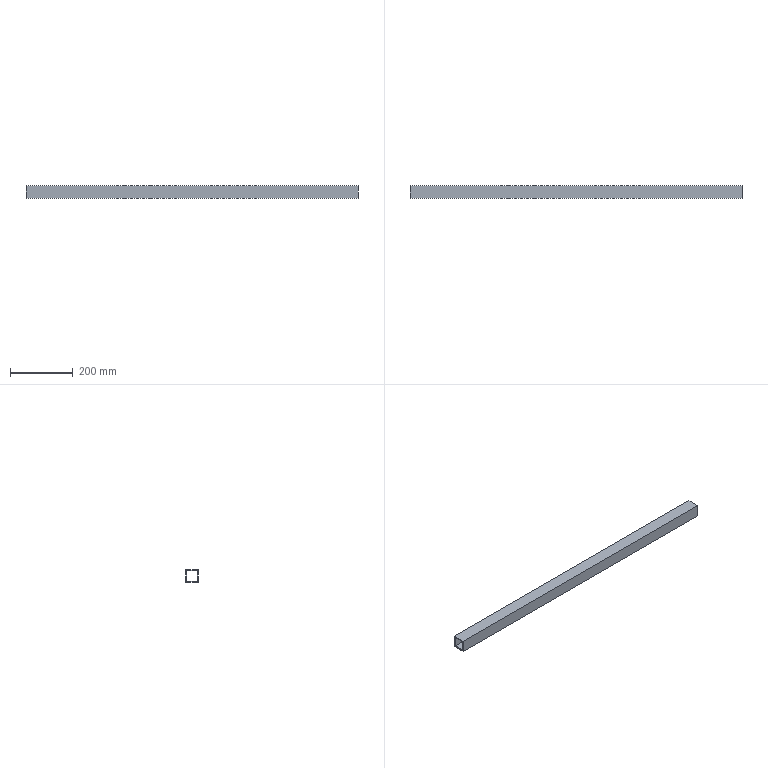Part | NX | features solid 2 | 1 solid | 10 faces | box 1060 x 40 x 40 mm | volume 610560 mm3 | plane 10
STEP:
#1=CARTESIAN_POINT('',(-1540.,-60.,-85.));
#2=VERTEX_POINT('',#1);
#3=CARTESIAN_POINT('',(-480.,-60.,-85.));
#4=VERTEX_POINT('',#3);
#5=CARTESIAN_POINT('',(119.393,-60.,-85.));
#6=DIRECTION('',(1.,0.,0.));
#7=VECTOR('',#6,1000.);
#8=LINE('',#5,#7);
#9=EDGE_CURVE('',#2,#4,#8,.T.);
#10=ORIENTED_EDGE('',*,*,#9,.T.);
#11=CARTESIAN_POINT('',(-480.,-60.,-45.));
#12=VERTEX_POINT('',#11);
#13=CARTESIAN_POINT('',(-480.,-60.,-70.));
#14=DIRECTION('',(0.,0.,1.));
#15=VECTOR('',#14,1000.);
#16=LINE('',#13,#15);
#17=EDGE_CURVE('',#4,#12,#16,.T.);
#18=ORIENTED_EDGE('',*,*,#17,.T.);
#19=CARTESIAN_POINT('',(-1540.,-60.,-45.));
#20=VERTEX_POINT('',#19);
#21=CARTESIAN_POINT('',(204.393,-60.,-45.));
#22=DIRECTION('',(1.,0.,0.));
#23=VECTOR('',#22,1000.);
#24=LINE('',#21,#23);
#25=EDGE_CURVE('',#20,#12,#24,.T.);
#26=ORIENTED_EDGE('',*,*,#25,.F.);
#27=CARTESIAN_POINT('',(-1540.,-60.,-70.));
#28=DIRECTION('',(0.,0.,-1.));
#29=VECTOR('',#28,1000.);
#30=LINE('',#27,#29);
#31=EDGE_CURVE('',#20,#2,#30,.T.);
#32=ORIENTED_EDGE('',*,*,#31,.T.);
#33=EDGE_LOOP('',(#10,#18,#26,#32));
#34=FACE_BOUND('',#33,.T.);
#35=CARTESIAN_POINT('',(119.393,-60.,-70.));
#36=DIRECTION('',(0.,1.,0.));
#37=DIRECTION('',(0.,0.,1.));
#38=AXIS2_PLACEMENT_3D('',#35,#36,#37);
#39=PLANE('',#38);
#40=ADVANCED_FACE('',(#34),#39,.F.);
#41=CARTESIAN_POINT('',(-1540.,-20.,-85.));
#42=VERTEX_POINT('',#41);
#43=CARTESIAN_POINT('',(-480.,-20.,-85.));
#44=VERTEX_POINT('',#43);
#45=CARTESIAN_POINT('',(204.393,-20.,-85.));
#46=DIRECTION('',(1.,0.,0.));
#47=VECTOR('',#46,1000.);
#48=LINE('',#45,#47);
#49=EDGE_CURVE('',#42,#44,#48,.T.);
#50=ORIENTED_EDGE('',*,*,#49,.T.);
#51=CARTESIAN_POINT('',(-480.,-640.,-85.));
#52=DIRECTION('',(0.,-1.,0.));
#53=VECTOR('',#52,1000.);
#54=LINE('',#51,#53);
#55=EDGE_CURVE('',#44,#4,#54,.T.);
#56=ORIENTED_EDGE('',*,*,#55,.T.);
#57=ORIENTED_EDGE('',*,*,#9,.F.);
#58=CARTESIAN_POINT('',(-1540.,-640.,-85.));
#59=DIRECTION('',(0.,1.,0.));
#60=VECTOR('',#59,1000.);
#61=LINE('',#58,#60);
#62=EDGE_CURVE('',#2,#42,#61,.T.);
#63=ORIENTED_EDGE('',*,*,#62,.T.);
#64=EDGE_LOOP('',(#50,#56,#57,#63));
#65=FACE_BOUND('',#64,.T.);
#66=CARTESIAN_POINT('',(204.393,-640.,-85.));
#67=DIRECTION('',(0.,0.,1.));
#68=DIRECTION('',(0.,-1.,0.));
#69=AXIS2_PLACEMENT_3D('',#66,#67,#68);
#70=PLANE('',#69);
#71=ADVANCED_FACE('',(#65),#70,.F.);
#72=ORIENTED_EDGE('',*,*,#25,.T.);
#73=CARTESIAN_POINT('',(-480.,-20.,-45.));
#74=VERTEX_POINT('',#73);
#75=CARTESIAN_POINT('',(-480.,-680.,-45.));
#76=DIRECTION('',(0.,1.,0.));
#77=VECTOR('',#76,1000.);
#78=LINE('',#75,#77);
#79=EDGE_CURVE('',#12,#74,#78,.T.);
#80=ORIENTED_EDGE('',*,*,#79,.T.);
#81=CARTESIAN_POINT('',(-1540.,-20.,-45.));
#82=VERTEX_POINT('',#81);
#83=CARTESIAN_POINT('',(204.393,-20.,-45.));
#84=DIRECTION('',(-1.,0.,0.));
#85=VECTOR('',#84,1000.);
#86=LINE('',#83,#85);
#87=EDGE_CURVE('',#74,#82,#86,.T.);
#88=ORIENTED_EDGE('',*,*,#87,.T.);
#89=CARTESIAN_POINT('',(-1540.,-680.,-45.));
#90=DIRECTION('',(0.,-1.,0.));
#91=VECTOR('',#90,1000.);
#92=LINE('',#89,#91);
#93=EDGE_CURVE('',#82,#20,#92,.T.);
#94=ORIENTED_EDGE('',*,*,#93,.T.);
#95=EDGE_LOOP('',(#72,#80,#88,#94));
#96=FACE_BOUND('',#95,.T.);
#97=CARTESIAN_POINT('',(204.393,-680.,-45.));
#98=DIRECTION('',(0.,0.,-1.));
#99=DIRECTION('',(0.,1.,0.));
#100=AXIS2_PLACEMENT_3D('',#97,#98,#99);
#101=PLANE('',#100);
#102=ADVANCED_FACE('',(#96),#101,.F.);
#103=ORIENTED_EDGE('',*,*,#87,.F.);
#104=CARTESIAN_POINT('',(-480.,-20.,-40.));
#105=DIRECTION('',(0.,0.,-1.));
#106=VECTOR('',#105,1000.);
#107=LINE('',#104,#106);
#108=EDGE_CURVE('',#74,#44,#107,.T.);
#109=ORIENTED_EDGE('',*,*,#108,.T.);
#110=ORIENTED_EDGE('',*,*,#49,.F.);
#111=CARTESIAN_POINT('',(-1540.,-20.,-40.));
#112=DIRECTION('',(0.,0.,1.));
#113=VECTOR('',#112,1000.);
#114=LINE('',#111,#113);
#115=EDGE_CURVE('',#42,#82,#114,.T.);
#116=ORIENTED_EDGE('',*,*,#115,.T.);
#117=EDGE_LOOP('',(#103,#109,#110,#116));
#118=FACE_BOUND('',#117,.T.);
#119=CARTESIAN_POINT('',(119.393,-20.,-40.));
#120=DIRECTION('',(0.,-1.,0.));
#121=DIRECTION('',(0.,0.,-1.));
#122=AXIS2_PLACEMENT_3D('',#119,#120,#121);
#123=PLANE('',#122);
#124=ADVANCED_FACE('',(#118),#123,.F.);
#125=CARTESIAN_POINT('',(-480.,-56.,-81.));
#126=VERTEX_POINT('',#125);
#127=CARTESIAN_POINT('',(-480.,-56.,-49.));
#128=VERTEX_POINT('',#127);
#129=CARTESIAN_POINT('',(-480.,-56.,-70.));
#130=DIRECTION('',(0.,0.,1.));
#131=VECTOR('',#130,1000.);
#132=LINE('',#129,#131);
#133=EDGE_CURVE('',#126,#128,#132,.T.);
#134=ORIENTED_EDGE('',*,*,#133,.F.);
#135=CARTESIAN_POINT('',(-1540.,-56.,-81.));
#136=VERTEX_POINT('',#135);
#137=CARTESIAN_POINT('',(119.393,-56.,-81.));
#138=DIRECTION('',(1.,0.,0.));
#139=VECTOR('',#138,1000.);
#140=LINE('',#137,#139);
#141=EDGE_CURVE('',#136,#126,#140,.T.);
#142=ORIENTED_EDGE('',*,*,#141,.F.);
#143=CARTESIAN_POINT('',(-1540.,-56.,-49.));
#144=VERTEX_POINT('',#143);
#145=CARTESIAN_POINT('',(-1540.,-56.,-70.));
#146=DIRECTION('',(0.,0.,-1.));
#147=VECTOR('',#146,1000.);
#148=LINE('',#145,#147);
#149=EDGE_CURVE('',#144,#136,#148,.T.);
#150=ORIENTED_EDGE('',*,*,#149,.F.);
#151=CARTESIAN_POINT('',(204.393,-56.,-49.));
#152=DIRECTION('',(1.,0.,0.));
#153=VECTOR('',#152,1000.);
#154=LINE('',#151,#153);
#155=EDGE_CURVE('',#144,#128,#154,.T.);
#156=ORIENTED_EDGE('',*,*,#155,.T.);
#157=EDGE_LOOP('',(#134,#142,#150,#156));
#158=FACE_BOUND('',#157,.T.);
#159=CARTESIAN_POINT('',(119.393,-56.,-70.));
#160=DIRECTION('',(0.,1.,0.));
#161=DIRECTION('',(0.,0.,1.));
#162=AXIS2_PLACEMENT_3D('',#159,#160,#161);
#163=PLANE('',#162);
#164=ADVANCED_FACE('',(#158),#163,.T.);
#165=CARTESIAN_POINT('',(-480.,-24.,-81.));
#166=VERTEX_POINT('',#165);
#167=CARTESIAN_POINT('',(-480.,-640.,-81.));
#168=DIRECTION('',(0.,-1.,0.));
#169=VECTOR('',#168,1000.);
#170=LINE('',#167,#169);
#171=EDGE_CURVE('',#166,#126,#170,.T.);
#172=ORIENTED_EDGE('',*,*,#171,.F.);
#173=CARTESIAN_POINT('',(-1540.,-24.,-81.));
#174=VERTEX_POINT('',#173);
#175=CARTESIAN_POINT('',(204.393,-24.,-81.));
#176=DIRECTION('',(1.,0.,0.));
#177=VECTOR('',#176,1000.);
#178=LINE('',#175,#177);
#179=EDGE_CURVE('',#174,#166,#178,.T.);
#180=ORIENTED_EDGE('',*,*,#179,.F.);
#181=CARTESIAN_POINT('',(-1540.,-640.,-81.));
#182=DIRECTION('',(0.,1.,0.));
#183=VECTOR('',#182,1000.);
#184=LINE('',#181,#183);
#185=EDGE_CURVE('',#136,#174,#184,.T.);
#186=ORIENTED_EDGE('',*,*,#185,.F.);
#187=ORIENTED_EDGE('',*,*,#141,.T.);
#188=EDGE_LOOP('',(#172,#180,#186,#187));
#189=FACE_BOUND('',#188,.T.);
#190=CARTESIAN_POINT('',(204.393,-640.,-81.));
#191=DIRECTION('',(0.,0.,1.));
#192=DIRECTION('',(0.,-1.,0.));
#193=AXIS2_PLACEMENT_3D('',#190,#191,#192);
#194=PLANE('',#193);
#195=ADVANCED_FACE('',(#189),#194,.T.);
#196=CARTESIAN_POINT('',(-480.,-24.,-49.));
#197=VERTEX_POINT('',#196);
#198=CARTESIAN_POINT('',(-480.,-680.,-49.));
#199=DIRECTION('',(0.,1.,0.));
#200=VECTOR('',#199,1000.);
#201=LINE('',#198,#200);
#202=EDGE_CURVE('',#128,#197,#201,.T.);
#203=ORIENTED_EDGE('',*,*,#202,.F.);
#204=ORIENTED_EDGE('',*,*,#155,.F.);
#205=CARTESIAN_POINT('',(-1540.,-24.,-49.));
#206=VERTEX_POINT('',#205);
#207=CARTESIAN_POINT('',(-1540.,-680.,-49.));
#208=DIRECTION('',(0.,-1.,0.));
#209=VECTOR('',#208,1000.);
#210=LINE('',#207,#209);
#211=EDGE_CURVE('',#206,#144,#210,.T.);
#212=ORIENTED_EDGE('',*,*,#211,.F.);
#213=CARTESIAN_POINT('',(204.393,-24.,-49.));
#214=DIRECTION('',(-1.,0.,0.));
#215=VECTOR('',#214,1000.);
#216=LINE('',#213,#215);
#217=EDGE_CURVE('',#197,#206,#216,.T.);
#218=ORIENTED_EDGE('',*,*,#217,.F.);
#219=EDGE_LOOP('',(#203,#204,#212,#218));
#220=FACE_BOUND('',#219,.T.);
#221=CARTESIAN_POINT('',(204.393,-680.,-49.));
#222=DIRECTION('',(0.,0.,-1.));
#223=DIRECTION('',(0.,1.,0.));
#224=AXIS2_PLACEMENT_3D('',#221,#222,#223);
#225=PLANE('',#224);
#226=ADVANCED_FACE('',(#220),#225,.T.);
#227=CARTESIAN_POINT('',(-480.,-24.,-40.));
#228=DIRECTION('',(0.,0.,-1.));
#229=VECTOR('',#228,1000.);
#230=LINE('',#227,#229);
#231=EDGE_CURVE('',#197,#166,#230,.T.);
#232=ORIENTED_EDGE('',*,*,#231,.F.);
#233=ORIENTED_EDGE('',*,*,#217,.T.);
#234=CARTESIAN_POINT('',(-1540.,-24.,-40.));
#235=DIRECTION('',(0.,0.,1.));
#236=VECTOR('',#235,1000.);
#237=LINE('',#234,#236);
#238=EDGE_CURVE('',#174,#206,#237,.T.);
#239=ORIENTED_EDGE('',*,*,#238,.F.);
#240=ORIENTED_EDGE('',*,*,#179,.T.);
#241=EDGE_LOOP('',(#232,#233,#239,#240));
#242=FACE_BOUND('',#241,.T.);
#243=CARTESIAN_POINT('',(119.393,-24.,-40.));
#244=DIRECTION('',(0.,-1.,0.));
#245=DIRECTION('',(0.,0.,-1.));
#246=AXIS2_PLACEMENT_3D('',#243,#244,#245);
#247=PLANE('',#246);
#248=ADVANCED_FACE('',(#242),#247,.T.);
#249=ORIENTED_EDGE('',*,*,#211,.T.);
#250=ORIENTED_EDGE('',*,*,#149,.T.);
#251=ORIENTED_EDGE('',*,*,#185,.T.);
#252=ORIENTED_EDGE('',*,*,#238,.T.);
#253=EDGE_LOOP('',(#249,#250,#251,#252));
#254=FACE_BOUND('',#253,.T.);
#255=ORIENTED_EDGE('',*,*,#31,.F.);
#256=ORIENTED_EDGE('',*,*,#93,.F.);
#257=ORIENTED_EDGE('',*,*,#115,.F.);
#258=ORIENTED_EDGE('',*,*,#62,.F.);
#259=EDGE_LOOP('',(#255,#256,#257,#258));
#260=FACE_BOUND('',#259,.T.);
#261=CARTESIAN_POINT('',(-1540.,490.,-39.5));
#262=DIRECTION('',(1.,0.,0.));
#263=DIRECTION('',(0.,-1.,0.));
#264=AXIS2_PLACEMENT_3D('',#261,#262,#263);
#265=PLANE('',#264);
#266=ADVANCED_FACE('',(#254,#260),#265,.F.);
#267=ORIENTED_EDGE('',*,*,#133,.T.);
#268=ORIENTED_EDGE('',*,*,#202,.T.);
#269=ORIENTED_EDGE('',*,*,#231,.T.);
#270=ORIENTED_EDGE('',*,*,#171,.T.);
#271=EDGE_LOOP('',(#267,#268,#269,#270));
#272=FACE_BOUND('',#271,.T.);
#273=ORIENTED_EDGE('',*,*,#55,.F.);
#274=ORIENTED_EDGE('',*,*,#108,.F.);
#275=ORIENTED_EDGE('',*,*,#79,.F.);
#276=ORIENTED_EDGE('',*,*,#17,.F.);
#277=EDGE_LOOP('',(#273,#274,#275,#276));
#278=FACE_BOUND('',#277,.T.);
#279=CARTESIAN_POINT('',(-480.,-30.4,2.));
#280=DIRECTION('',(-1.,0.,0.));
#281=DIRECTION('',(0.,0.,1.));
#282=AXIS2_PLACEMENT_3D('',#279,#280,#281);
#283=PLANE('',#282);
#284=ADVANCED_FACE('',(#272,#278),#283,.F.);
#285=CLOSED_SHELL('',(#40,#71,#102,#124,#164,#195,#226,#248,#266,#284));
#286=MANIFOLD_SOLID_BREP('',#285);
#287=(LENGTH_UNIT()NAMED_UNIT(*)SI_UNIT(.MILLI.,.METRE.));
#288=UNCERTAINTY_MEASURE_WITH_UNIT(LENGTH_MEASURE(0.00001),#287,'','');
#289=(NAMED_UNIT(*)PLANE_ANGLE_UNIT()SI_UNIT($,.RADIAN.));
#290=(NAMED_UNIT(*)SI_UNIT($,.STERADIAN.)SOLID_ANGLE_UNIT());
#291=(GEOMETRIC_REPRESENTATION_CONTEXT(3)GLOBAL_UNCERTAINTY_ASSIGNED_CONTEXT((#288))GLOBAL_UNIT_ASSIGNED_CONTEXT((#287,#289,#290))REPRESENTATION_CONTEXT('',''));
#292=ADVANCED_BREP_SHAPE_REPRESENTATION('',(#286),#291);